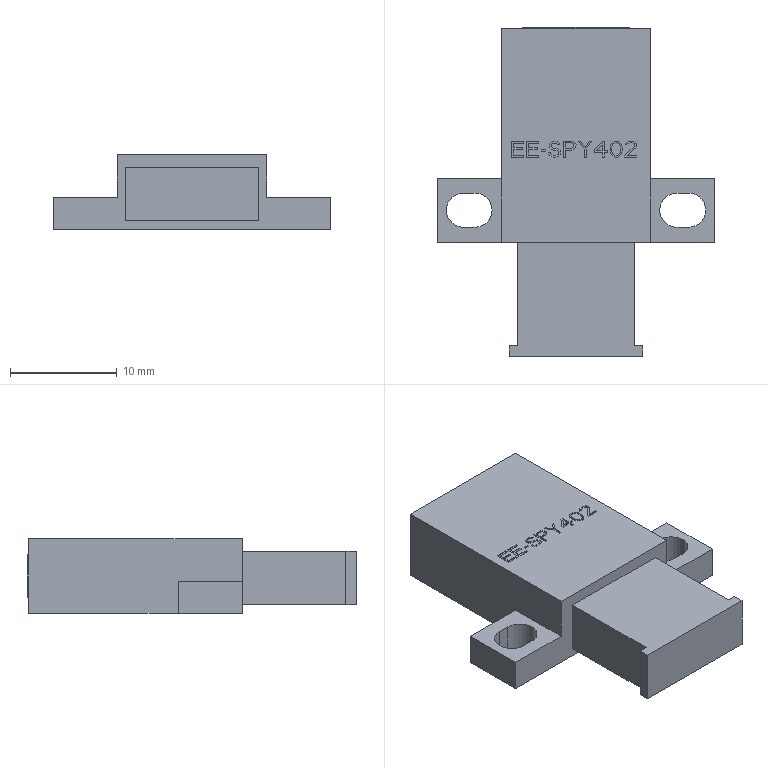Part | NX | 1 solid | 249 faces | box 26 x 30.8 x 7 mm | volume 2702 mm3 | plane 243 | cylinder 6 | commonest cylinder face diameters 3.2 x6